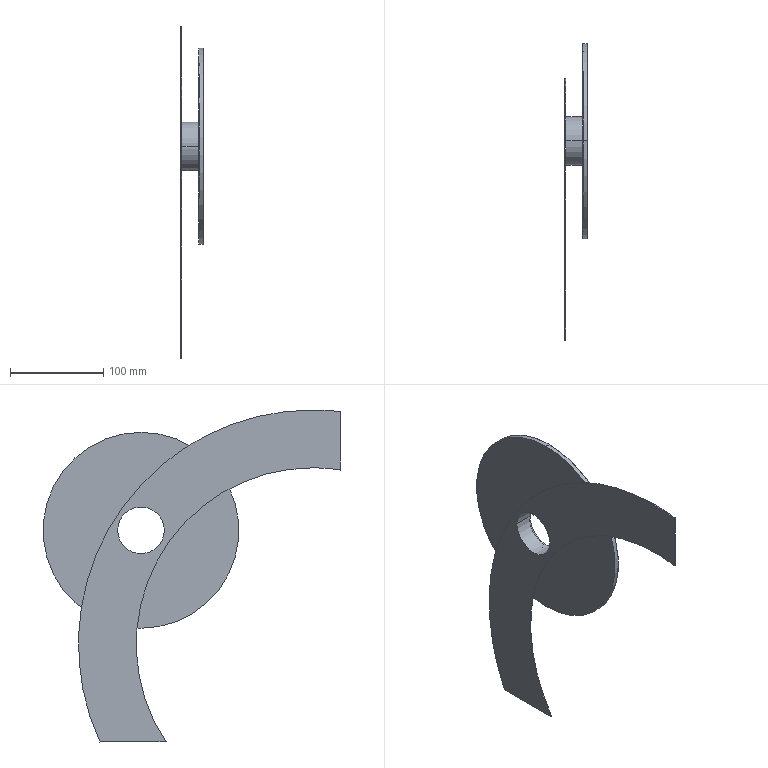Part | STEP file | 09-24 Track cover plate | 1 solid | 19 faces | box 24 x 319 x 356 mm | volume 66305 mm3 | cylinder 12 | plane 7 | commonest cylinder face diameters 50 x2 52 x2 208 x2 210 x2 378 x2 502 x2
STEP:
#1=CARTESIAN_POINT('',(0.,0.,0.));
#2=DIRECTION('',(0.,0.,1.));
#3=DIRECTION('',(1.,0.,0.));
#4=AXIS2_PLACEMENT_3D('',#1,#2,#3);
#5=CARTESIAN_POINT('',(24.,184.,226.));
#6=VERTEX_POINT('',#5);
#7=CARTESIAN_POINT('',(20.,184.,226.));
#8=VERTEX_POINT('',#7);
#9=CARTESIAN_POINT('',(24.,184.,226.));
#10=DIRECTION('',(-1.,0.,0.));
#11=VECTOR('',#10,1.);
#12=LINE('',#9,#11);
#13=CARTESIAN_POINT('',(24.,184.,122.));
#14=DIRECTION('',(-1.,0.,0.));
#15=DIRECTION('',(0.,0.,1.));
#16=AXIS2_PLACEMENT_3D('',#13,#14,#15);
#17=CYLINDRICAL_SURFACE('',#16,104.);
#18=CARTESIAN_POINT('',(6.283,0.));
#19=DIRECTION('',(0.,1.));
#20=VECTOR('',#19,1.);
#21=LINE('',#18,#20);
#22=(GEOMETRIC_REPRESENTATION_CONTEXT(2)PARAMETRIC_REPRESENTATION_CONTEXT()REPRESENTATION_CONTEXT('',''));
#23=DEFINITIONAL_REPRESENTATION('',(#21),#22);
#24=PCURVE('',#17,#23);
#25=CARTESIAN_POINT('',(24.,184.,122.));
#26=DIRECTION('',(-1.,0.,0.));
#27=DIRECTION('',(0.,0.,1.));
#28=AXIS2_PLACEMENT_3D('',#25,#26,#27);
#29=CYLINDRICAL_SURFACE('',#28,104.);
#30=CARTESIAN_POINT('',(0.,0.));
#31=DIRECTION('',(0.,1.));
#32=VECTOR('',#31,1.);
#33=LINE('',#30,#32);
#34=(GEOMETRIC_REPRESENTATION_CONTEXT(2)PARAMETRIC_REPRESENTATION_CONTEXT()REPRESENTATION_CONTEXT('',''));
#35=DEFINITIONAL_REPRESENTATION('',(#33),#34);
#36=PCURVE('',#29,#35);
#37=SURFACE_CURVE('',#12,(#24,#36),.PCURVE_S1.);
#38=EDGE_CURVE('',#6,#8,#37,.T.);
#39=ORIENTED_EDGE('',*,*,#38,.T.);
#40=CARTESIAN_POINT('',(20.,184.,18.));
#41=VERTEX_POINT('',#40);
#42=CARTESIAN_POINT('',(20.,184.,122.));
#43=DIRECTION('',(-1.,0.,0.));
#44=DIRECTION('',(0.,0.,1.));
#45=AXIS2_PLACEMENT_3D('',#42,#43,#44);
#46=CIRCLE('',#45,104.);
#47=CARTESIAN_POINT('',(0.,4.));
#48=DIRECTION('',(1.,0.));
#49=VECTOR('',#48,1.);
#50=LINE('',#47,#49);
#51=(GEOMETRIC_REPRESENTATION_CONTEXT(2)PARAMETRIC_REPRESENTATION_CONTEXT()REPRESENTATION_CONTEXT('',''));
#52=DEFINITIONAL_REPRESENTATION('',(#50),#51);
#53=PCURVE('',#17,#52);
#54=CARTESIAN_POINT('',(20.,78.752,227.248));
#55=DIRECTION('',(1.,0.,0.));
#56=DIRECTION('',(0.,0.,-1.));
#57=AXIS2_PLACEMENT_3D('',#54,#55,#56);
#58=PLANE('',#57);
#59=CARTESIAN_POINT('',(1.248,105.248));
#60=CARTESIAN_POINT('',(1.248,285.381));
#61=CARTESIAN_POINT('',(157.248,195.315));
#62=CARTESIAN_POINT('',(313.248,105.248));
#63=CARTESIAN_POINT('',(157.248,15.181));
#64=CARTESIAN_POINT('',(1.248,-74.885));
#65=CARTESIAN_POINT('',(1.248,105.248));
#66=(BOUNDED_CURVE()B_SPLINE_CURVE(2,(#59,#60,#61,#62,#63,#64,#65),.UNSPECIFIED.,.T.,.F.)B_SPLINE_CURVE_WITH_KNOTS((1,2,2,2,2,1),(-2.094,0.,2.094,4.189,6.283,8.378),.UNSPECIFIED.)CURVE()GEOMETRIC_REPRESENTATION_ITEM()RATIONAL_B_SPLINE_CURVE((1.,0.5,1.,0.5,1.,0.5,1.))REPRESENTATION_ITEM(''));
#67=(GEOMETRIC_REPRESENTATION_CONTEXT(2)PARAMETRIC_REPRESENTATION_CONTEXT()REPRESENTATION_CONTEXT('',''));
#68=DEFINITIONAL_REPRESENTATION('',(#66),#67);
#69=PCURVE('',#58,#68);
#70=SURFACE_CURVE('',#46,(#53,#69),.PCURVE_S1.);
#71=EDGE_CURVE('',#41,#8,#70,.T.);
#72=ORIENTED_EDGE('',*,*,#71,.F.);
#73=CARTESIAN_POINT('',(24.,184.,18.));
#74=VERTEX_POINT('',#73);
#75=CARTESIAN_POINT('',(24.,184.,18.));
#76=DIRECTION('',(-1.,0.,0.));
#77=VECTOR('',#76,1.);
#78=LINE('',#75,#77);
#79=CARTESIAN_POINT('',(3.142,0.));
#80=DIRECTION('',(0.,1.));
#81=VECTOR('',#80,1.);
#82=LINE('',#79,#81);
#83=(GEOMETRIC_REPRESENTATION_CONTEXT(2)PARAMETRIC_REPRESENTATION_CONTEXT()REPRESENTATION_CONTEXT('',''));
#84=DEFINITIONAL_REPRESENTATION('',(#82),#83);
#85=PCURVE('',#17,#84);
#86=CARTESIAN_POINT('',(3.142,0.));
#87=DIRECTION('',(0.,1.));
#88=VECTOR('',#87,1.);
#89=LINE('',#86,#88);
#90=(GEOMETRIC_REPRESENTATION_CONTEXT(2)PARAMETRIC_REPRESENTATION_CONTEXT()REPRESENTATION_CONTEXT('',''));
#91=DEFINITIONAL_REPRESENTATION('',(#89),#90);
#92=PCURVE('',#29,#91);
#93=SURFACE_CURVE('',#78,(#85,#92),.PCURVE_S1.);
#94=EDGE_CURVE('',#74,#41,#93,.T.);
#95=ORIENTED_EDGE('',*,*,#94,.F.);
#96=CARTESIAN_POINT('',(24.,184.,122.));
#97=DIRECTION('',(1.,0.,0.));
#98=DIRECTION('',(0.,0.,1.));
#99=AXIS2_PLACEMENT_3D('',#96,#97,#98);
#100=CIRCLE('',#99,104.);
#101=CARTESIAN_POINT('',(6.283,0.));
#102=DIRECTION('',(-1.,0.));
#103=VECTOR('',#102,1.);
#104=LINE('',#101,#103);
#105=(GEOMETRIC_REPRESENTATION_CONTEXT(2)PARAMETRIC_REPRESENTATION_CONTEXT()REPRESENTATION_CONTEXT('',''));
#106=DEFINITIONAL_REPRESENTATION('',(#104),#105);
#107=PCURVE('',#17,#106);
#108=CARTESIAN_POINT('',(24.,77.74,228.26));
#109=DIRECTION('',(1.,0.,0.));
#110=DIRECTION('',(0.,0.,-1.));
#111=AXIS2_PLACEMENT_3D('',#108,#109,#110);
#112=PLANE('',#111);
#113=CARTESIAN_POINT('',(106.26,106.26));
#114=DIRECTION('',(-1.,0.));
#115=AXIS2_PLACEMENT_2D('',#113,#114);
#116=CIRCLE('',#115,104.);
#117=(GEOMETRIC_REPRESENTATION_CONTEXT(2)PARAMETRIC_REPRESENTATION_CONTEXT()REPRESENTATION_CONTEXT('',''));
#118=DEFINITIONAL_REPRESENTATION('',(#116),#117);
#119=PCURVE('',#112,#118);
#120=SURFACE_CURVE('',#100,(#107,#119),.PCURVE_S1.);
#121=EDGE_CURVE('',#6,#74,#120,.T.);
#122=ORIENTED_EDGE('',*,*,#121,.F.);
#123=EDGE_LOOP('',(#39,#72,#95,#122));
#124=FACE_BOUND('',#123,.F.);
#125=ADVANCED_FACE('',(#124),#17,.F.);
#126=CARTESIAN_POINT('',(20.,159.,122.));
#127=VERTEX_POINT('',#126);
#128=CARTESIAN_POINT('',(0.,159.,122.));
#129=VERTEX_POINT('',#128);
#130=CARTESIAN_POINT('',(20.,159.,122.));
#131=DIRECTION('',(-1.,0.,0.));
#132=VECTOR('',#131,1.);
#133=LINE('',#130,#132);
#134=CARTESIAN_POINT('',(20.,184.,122.));
#135=DIRECTION('',(-1.,0.,0.));
#136=DIRECTION('',(0.,-1.,0.));
#137=AXIS2_PLACEMENT_3D('',#134,#135,#136);
#138=CYLINDRICAL_SURFACE('',#137,25.);
#139=CARTESIAN_POINT('',(6.283,0.));
#140=DIRECTION('',(0.,1.));
#141=VECTOR('',#140,1.);
#142=LINE('',#139,#141);
#143=(GEOMETRIC_REPRESENTATION_CONTEXT(2)PARAMETRIC_REPRESENTATION_CONTEXT()REPRESENTATION_CONTEXT('',''));
#144=DEFINITIONAL_REPRESENTATION('',(#142),#143);
#145=PCURVE('',#138,#144);
#146=CARTESIAN_POINT('',(20.,184.,122.));
#147=DIRECTION('',(-1.,0.,0.));
#148=DIRECTION('',(0.,-1.,0.));
#149=AXIS2_PLACEMENT_3D('',#146,#147,#148);
#150=CYLINDRICAL_SURFACE('',#149,25.);
#151=CARTESIAN_POINT('',(0.,0.));
#152=DIRECTION('',(0.,1.));
#153=VECTOR('',#152,1.);
#154=LINE('',#151,#153);
#155=(GEOMETRIC_REPRESENTATION_CONTEXT(2)PARAMETRIC_REPRESENTATION_CONTEXT()REPRESENTATION_CONTEXT('',''));
#156=DEFINITIONAL_REPRESENTATION('',(#154),#155);
#157=PCURVE('',#150,#156);
#158=SURFACE_CURVE('',#133,(#145,#157),.PCURVE_S1.);
#159=EDGE_CURVE('',#127,#129,#158,.T.);
#160=ORIENTED_EDGE('',*,*,#159,.T.);
#161=CARTESIAN_POINT('',(0.,209.,122.));
#162=VERTEX_POINT('',#161);
#163=CARTESIAN_POINT('',(0.,184.,122.));
#164=DIRECTION('',(-1.,0.,0.));
#165=DIRECTION('',(0.,-1.,0.));
#166=AXIS2_PLACEMENT_3D('',#163,#164,#165);
#167=CIRCLE('',#166,25.);
#168=CARTESIAN_POINT('',(0.,20.));
#169=DIRECTION('',(1.,0.));
#170=VECTOR('',#169,1.);
#171=LINE('',#168,#170);
#172=(GEOMETRIC_REPRESENTATION_CONTEXT(2)PARAMETRIC_REPRESENTATION_CONTEXT()REPRESENTATION_CONTEXT('',''));
#173=DEFINITIONAL_REPRESENTATION('',(#171),#172);
#174=PCURVE('',#138,#173);
#175=CARTESIAN_POINT('',(0.,-30.,253.136));
#176=DIRECTION('',(1.,0.,0.));
#177=DIRECTION('',(0.,0.,-1.));
#178=AXIS2_PLACEMENT_3D('',#175,#176,#177);
#179=PLANE('',#178);
#180=CARTESIAN_POINT('',(131.136,189.));
#181=CARTESIAN_POINT('',(87.835,189.));
#182=CARTESIAN_POINT('',(109.485,226.5));
#183=CARTESIAN_POINT('',(131.136,264.));
#184=CARTESIAN_POINT('',(152.787,226.5));
#185=CARTESIAN_POINT('',(174.437,189.));
#186=CARTESIAN_POINT('',(131.136,189.));
#187=(BOUNDED_CURVE()B_SPLINE_CURVE(2,(#180,#181,#182,#183,#184,#185,#186),.UNSPECIFIED.,.T.,.F.)B_SPLINE_CURVE_WITH_KNOTS((1,2,2,2,2,1),(-2.094,0.,2.094,4.189,6.283,8.378),.UNSPECIFIED.)CURVE()GEOMETRIC_REPRESENTATION_ITEM()RATIONAL_B_SPLINE_CURVE((1.,0.5,1.,0.5,1.,0.5,1.))REPRESENTATION_ITEM(''));
#188=(GEOMETRIC_REPRESENTATION_CONTEXT(2)PARAMETRIC_REPRESENTATION_CONTEXT()REPRESENTATION_CONTEXT('',''));
#189=DEFINITIONAL_REPRESENTATION('',(#187),#188);
#190=PCURVE('',#179,#189);
#191=SURFACE_CURVE('',#167,(#174,#190),.PCURVE_S1.);
#192=EDGE_CURVE('',#162,#129,#191,.T.);
#193=ORIENTED_EDGE('',*,*,#192,.F.);
#194=CARTESIAN_POINT('',(20.,209.,122.));
#195=VERTEX_POINT('',#194);
#196=CARTESIAN_POINT('',(20.,209.,122.));
#197=DIRECTION('',(-1.,0.,0.));
#198=VECTOR('',#197,1.);
#199=LINE('',#196,#198);
#200=CARTESIAN_POINT('',(3.142,0.));
#201=DIRECTION('',(0.,1.));
#202=VECTOR('',#201,1.);
#203=LINE('',#200,#202);
#204=(GEOMETRIC_REPRESENTATION_CONTEXT(2)PARAMETRIC_REPRESENTATION_CONTEXT()REPRESENTATION_CONTEXT('',''));
#205=DEFINITIONAL_REPRESENTATION('',(#203),#204);
#206=PCURVE('',#138,#205);
#207=CARTESIAN_POINT('',(3.142,0.));
#208=DIRECTION('',(0.,1.));
#209=VECTOR('',#208,1.);
#210=LINE('',#207,#209);
#211=(GEOMETRIC_REPRESENTATION_CONTEXT(2)PARAMETRIC_REPRESENTATION_CONTEXT()REPRESENTATION_CONTEXT('',''));
#212=DEFINITIONAL_REPRESENTATION('',(#210),#211);
#213=PCURVE('',#150,#212);
#214=SURFACE_CURVE('',#199,(#206,#213),.PCURVE_S1.);
#215=EDGE_CURVE('',#195,#162,#214,.T.);
#216=ORIENTED_EDGE('',*,*,#215,.F.);
#217=CARTESIAN_POINT('',(20.,184.,122.));
#218=DIRECTION('',(-1.,0.,0.));
#219=DIRECTION('',(0.,-1.,0.));
#220=AXIS2_PLACEMENT_3D('',#217,#218,#219);
#221=CIRCLE('',#220,25.);
#222=CARTESIAN_POINT('',(0.,0.));
#223=DIRECTION('',(1.,0.));
#224=VECTOR('',#223,1.);
#225=LINE('',#222,#224);
#226=(GEOMETRIC_REPRESENTATION_CONTEXT(2)PARAMETRIC_REPRESENTATION_CONTEXT()REPRESENTATION_CONTEXT('',''));
#227=DEFINITIONAL_REPRESENTATION('',(#225),#226);
#228=PCURVE('',#138,#227);
#229=CARTESIAN_POINT('',(105.248,80.248));
#230=CARTESIAN_POINT('',(61.947,80.248));
#231=CARTESIAN_POINT('',(83.597,117.748));
#232=CARTESIAN_POINT('',(105.248,155.248));
#233=CARTESIAN_POINT('',(126.899,117.748));
#234=CARTESIAN_POINT('',(148.549,80.248));
#235=CARTESIAN_POINT('',(105.248,80.248));
#236=(BOUNDED_CURVE()B_SPLINE_CURVE(2,(#229,#230,#231,#232,#233,#234,#235),.UNSPECIFIED.,.T.,.F.)B_SPLINE_CURVE_WITH_KNOTS((1,2,2,2,2,1),(-2.094,0.,2.094,4.189,6.283,8.378),.UNSPECIFIED.)CURVE()GEOMETRIC_REPRESENTATION_ITEM()RATIONAL_B_SPLINE_CURVE((1.,0.5,1.,0.5,1.,0.5,1.))REPRESENTATION_ITEM(''));
#237=(GEOMETRIC_REPRESENTATION_CONTEXT(2)PARAMETRIC_REPRESENTATION_CONTEXT()REPRESENTATION_CONTEXT('',''));
#238=DEFINITIONAL_REPRESENTATION('',(#236),#237);
#239=PCURVE('',#58,#238);
#240=SURFACE_CURVE('',#221,(#228,#239),.PCURVE_S1.);
#241=EDGE_CURVE('',#195,#127,#240,.T.);
#242=ORIENTED_EDGE('',*,*,#241,.T.);
#243=EDGE_LOOP('',(#160,#193,#216,#242));
#244=FACE_BOUND('',#243,.F.);
#245=ADVANCED_FACE('',(#244),#138,.F.);
#246=CARTESIAN_POINT('',(19.,184.,227.));
#247=VERTEX_POINT('',#246);
#248=CARTESIAN_POINT('',(19.,184.,17.));
#249=VERTEX_POINT('',#248);
#250=CARTESIAN_POINT('',(19.,184.,122.));
#251=DIRECTION('',(-1.,0.,0.));
#252=DIRECTION('',(0.,0.,-1.));
#253=AXIS2_PLACEMENT_3D('',#250,#251,#252);
#254=CIRCLE('',#253,105.);
#255=CARTESIAN_POINT('',(19.,184.,122.));
#256=DIRECTION('',(1.,0.,0.));
#257=DIRECTION('',(0.,0.,-1.));
#258=AXIS2_PLACEMENT_3D('',#255,#256,#257);
#259=CYLINDRICAL_SURFACE('',#258,105.);
#260=CARTESIAN_POINT('',(6.283,0.));
#261=DIRECTION('',(-1.,0.));
#262=VECTOR('',#261,1.);
#263=LINE('',#260,#262);
#264=(GEOMETRIC_REPRESENTATION_CONTEXT(2)PARAMETRIC_REPRESENTATION_CONTEXT()REPRESENTATION_CONTEXT('',''));
#265=DEFINITIONAL_REPRESENTATION('',(#263),#264);
#266=PCURVE('',#259,#265);
#267=CARTESIAN_POINT('',(19.,77.74,228.26));
#268=DIRECTION('',(1.,0.,0.));
#269=DIRECTION('',(0.,0.,-1.));
#270=AXIS2_PLACEMENT_3D('',#267,#268,#269);
#271=PLANE('',#270);
#272=CARTESIAN_POINT('',(211.26,106.26));
#273=CARTESIAN_POINT('',(211.26,-75.605));
#274=CARTESIAN_POINT('',(53.76,15.327));
#275=CARTESIAN_POINT('',(-103.74,106.26));
#276=CARTESIAN_POINT('',(53.76,197.193));
#277=CARTESIAN_POINT('',(211.26,288.125));
#278=CARTESIAN_POINT('',(211.26,106.26));
#279=(BOUNDED_CURVE()B_SPLINE_CURVE(2,(#272,#273,#274,#275,#276,#277,#278),.UNSPECIFIED.,.T.,.F.)B_SPLINE_CURVE_WITH_KNOTS((1,2,2,2,2,1),(-2.094,0.,2.094,4.189,6.283,8.378),.UNSPECIFIED.)CURVE()GEOMETRIC_REPRESENTATION_ITEM()RATIONAL_B_SPLINE_CURVE((1.,0.5,1.,0.5,1.,0.5,1.))REPRESENTATION_ITEM(''));
#280=(GEOMETRIC_REPRESENTATION_CONTEXT(2)PARAMETRIC_REPRESENTATION_CONTEXT()REPRESENTATION_CONTEXT('',''));
#281=DEFINITIONAL_REPRESENTATION('',(#279),#280);
#282=PCURVE('',#271,#281);
#283=SURFACE_CURVE('',#254,(#266,#282),.PCURVE_S1.);
#284=EDGE_CURVE('',#247,#249,#283,.T.);
#285=ORIENTED_EDGE('',*,*,#284,.F.);
#286=CARTESIAN_POINT('',(24.,184.,227.));
#287=VERTEX_POINT('',#286);
#288=CARTESIAN_POINT('',(19.,184.,227.));
#289=DIRECTION('',(1.,0.,0.));
#290=VECTOR('',#289,1.);
#291=LINE('',#288,#290);
#292=CARTESIAN_POINT('',(3.142,0.));
#293=DIRECTION('',(0.,1.));
#294=VECTOR('',#293,1.);
#295=LINE('',#292,#294);
#296=(GEOMETRIC_REPRESENTATION_CONTEXT(2)PARAMETRIC_REPRESENTATION_CONTEXT()REPRESENTATION_CONTEXT('',''));
#297=DEFINITIONAL_REPRESENTATION('',(#295),#296);
#298=PCURVE('',#259,#297);
#299=CARTESIAN_POINT('',(19.,184.,122.));
#300=DIRECTION('',(1.,0.,0.));
#301=DIRECTION('',(0.,0.,-1.));
#302=AXIS2_PLACEMENT_3D('',#299,#300,#301);
#303=CYLINDRICAL_SURFACE('',#302,105.);
#304=CARTESIAN_POINT('',(3.142,0.));
#305=DIRECTION('',(0.,1.));
#306=VECTOR('',#305,1.);
#307=LINE('',#304,#306);
#308=(GEOMETRIC_REPRESENTATION_CONTEXT(2)PARAMETRIC_REPRESENTATION_CONTEXT()REPRESENTATION_CONTEXT('',''));
#309=DEFINITIONAL_REPRESENTATION('',(#307),#308);
#310=PCURVE('',#303,#309);
#311=SURFACE_CURVE('',#291,(#298,#310),.PCURVE_S1.);
#312=EDGE_CURVE('',#247,#287,#311,.T.);
#313=ORIENTED_EDGE('',*,*,#312,.T.);
#314=CARTESIAN_POINT('',(24.,184.,17.));
#315=VERTEX_POINT('',#314);
#316=CARTESIAN_POINT('',(24.,184.,122.));
#317=DIRECTION('',(1.,0.,0.));
#318=DIRECTION('',(0.,0.,-1.));
#319=AXIS2_PLACEMENT_3D('',#316,#317,#318);
#320=CIRCLE('',#319,105.);
#321=CARTESIAN_POINT('',(0.,5.));
#322=DIRECTION('',(1.,0.));
#323=VECTOR('',#322,1.);
#324=LINE('',#321,#323);
#325=(GEOMETRIC_REPRESENTATION_CONTEXT(2)PARAMETRIC_REPRESENTATION_CONTEXT()REPRESENTATION_CONTEXT('',''));
#326=DEFINITIONAL_REPRESENTATION('',(#324),#325);
#327=PCURVE('',#259,#326);
#328=CARTESIAN_POINT('',(106.26,106.26));
#329=DIRECTION('',(1.,0.));
#330=AXIS2_PLACEMENT_2D('',#328,#329);
#331=CIRCLE('',#330,105.);
#332=(GEOMETRIC_REPRESENTATION_CONTEXT(2)PARAMETRIC_REPRESENTATION_CONTEXT()REPRESENTATION_CONTEXT('',''));
#333=DEFINITIONAL_REPRESENTATION('',(#331),#332);
#334=PCURVE('',#112,#333);
#335=SURFACE_CURVE('',#320,(#327,#334),.PCURVE_S1.);
#336=EDGE_CURVE('',#315,#287,#335,.T.);
#337=ORIENTED_EDGE('',*,*,#336,.F.);
#338=CARTESIAN_POINT('',(19.,184.,17.));
#339=DIRECTION('',(1.,0.,0.));
#340=VECTOR('',#339,1.);
#341=LINE('',#338,#340);
#342=CARTESIAN_POINT('',(0.,0.));
#343=DIRECTION('',(0.,1.));
#344=VECTOR('',#343,1.);
#345=LINE('',#342,#344);
#346=(GEOMETRIC_REPRESENTATION_CONTEXT(2)PARAMETRIC_REPRESENTATION_CONTEXT()REPRESENTATION_CONTEXT('',''));
#347=DEFINITIONAL_REPRESENTATION('',(#345),#346);
#348=PCURVE('',#259,#347);
#349=CARTESIAN_POINT('',(6.283,0.));
#350=DIRECTION('',(0.,1.));
#351=VECTOR('',#350,1.);
#352=LINE('',#349,#351);
#353=(GEOMETRIC_REPRESENTATION_CONTEXT(2)PARAMETRIC_REPRESENTATION_CONTEXT()REPRESENTATION_CONTEXT('',''));
#354=DEFINITIONAL_REPRESENTATION('',(#352),#353);
#355=PCURVE('',#303,#354);
#356=SURFACE_CURVE('',#341,(#348,#355),.PCURVE_S1.);
#357=EDGE_CURVE('',#249,#315,#356,.T.);
#358=ORIENTED_EDGE('',*,*,#357,.F.);
#359=EDGE_LOOP('',(#285,#313,#337,#358));
#360=FACE_BOUND('',#359,.T.);
#361=ADVANCED_FACE('',(#360),#259,.T.);
#362=CARTESIAN_POINT('',(1.,0.,251.));
#363=VERTEX_POINT('',#362);
#364=CARTESIAN_POINT('',(1.,-30.,249.201));
#365=VERTEX_POINT('',#364);
#366=CARTESIAN_POINT('',(1.,0.,0.));
#367=DIRECTION('',(1.,0.,0.));
#368=DIRECTION('',(0.,0.,1.));
#369=AXIS2_PLACEMENT_3D('',#366,#367,#368);
#370=CIRCLE('',#369,251.);
#371=CARTESIAN_POINT('',(1.,0.,0.));
#372=DIRECTION('',(-1.,0.,0.));
#373=DIRECTION('',(0.,0.,1.));
#374=AXIS2_PLACEMENT_3D('',#371,#372,#373);
#375=CYLINDRICAL_SURFACE('',#374,251.);
#376=CARTESIAN_POINT('',(6.283,0.));
#377=DIRECTION('',(-1.,0.));
#378=VECTOR('',#377,1.);
#379=LINE('',#376,#378);
#380=(GEOMETRIC_REPRESENTATION_CONTEXT(2)PARAMETRIC_REPRESENTATION_CONTEXT()REPRESENTATION_CONTEXT('',''));
#381=DEFINITIONAL_REPRESENTATION('',(#379),#380);
#382=PCURVE('',#375,#381);
#383=CARTESIAN_POINT('',(1.,-30.,253.136));
#384=DIRECTION('',(1.,0.,0.));
#385=DIRECTION('',(0.,0.,-1.));
#386=AXIS2_PLACEMENT_3D('',#383,#384,#385);
#387=PLANE('',#386);
#388=CARTESIAN_POINT('',(253.136,30.));
#389=DIRECTION('',(-1.,0.));
#390=AXIS2_PLACEMENT_2D('',#388,#389);
#391=CIRCLE('',#390,251.);
#392=(GEOMETRIC_REPRESENTATION_CONTEXT(2)PARAMETRIC_REPRESENTATION_CONTEXT()REPRESENTATION_CONTEXT('',''));
#393=DEFINITIONAL_REPRESENTATION('',(#391),#392);
#394=PCURVE('',#387,#393);
#395=SURFACE_CURVE('',#370,(#382,#394),.PCURVE_S1.);
#396=EDGE_CURVE('',#363,#365,#395,.T.);
#397=ORIENTED_EDGE('',*,*,#396,.F.);
#398=CARTESIAN_POINT('',(0.,0.,251.));
#399=VERTEX_POINT('',#398);
#400=CARTESIAN_POINT('',(1.,0.,251.));
#401=DIRECTION('',(-1.,0.,0.));
#402=VECTOR('',#401,1.);
#403=LINE('',#400,#402);
#404=CARTESIAN_POINT('',(6.283,0.));
#405=DIRECTION('',(0.,1.));
#406=VECTOR('',#405,1.);
#407=LINE('',#404,#406);
#408=(GEOMETRIC_REPRESENTATION_CONTEXT(2)PARAMETRIC_REPRESENTATION_CONTEXT()REPRESENTATION_CONTEXT('',''));
#409=DEFINITIONAL_REPRESENTATION('',(#407),#408);
#410=PCURVE('',#375,#409);
#411=CARTESIAN_POINT('',(1.,0.,0.));
#412=DIRECTION('',(-1.,0.,0.));
#413=DIRECTION('',(0.,0.,1.));
#414=AXIS2_PLACEMENT_3D('',#411,#412,#413);
#415=CYLINDRICAL_SURFACE('',#414,251.);
#416=CARTESIAN_POINT('',(0.,0.));
#417=DIRECTION('',(0.,1.));
#418=VECTOR('',#417,1.);
#419=LINE('',#416,#418);
#420=(GEOMETRIC_REPRESENTATION_CONTEXT(2)PARAMETRIC_REPRESENTATION_CONTEXT()REPRESENTATION_CONTEXT('',''));
#421=DEFINITIONAL_REPRESENTATION('',(#419),#420);
#422=PCURVE('',#415,#421);
#423=SURFACE_CURVE('',#403,(#410,#422),.PCURVE_S1.);
#424=EDGE_CURVE('',#363,#399,#423,.T.);
#425=ORIENTED_EDGE('',*,*,#424,.T.);
#426=CARTESIAN_POINT('',(0.,-30.,249.201));
#427=VERTEX_POINT('',#426);
#428=CARTESIAN_POINT('',(0.,0.,0.));
#429=DIRECTION('',(1.,0.,0.));
#430=DIRECTION('',(0.,0.,1.));
#431=AXIS2_PLACEMENT_3D('',#428,#429,#430);
#432=CIRCLE('',#431,251.);
#433=CARTESIAN_POINT('',(6.283,1.));
#434=DIRECTION('',(-1.,0.));
#435=VECTOR('',#434,1.);
#436=LINE('',#433,#435);
#437=(GEOMETRIC_REPRESENTATION_CONTEXT(2)PARAMETRIC_REPRESENTATION_CONTEXT()REPRESENTATION_CONTEXT('',''));
#438=DEFINITIONAL_REPRESENTATION('',(#436),#437);
#439=PCURVE('',#375,#438);
#440=CARTESIAN_POINT('',(253.136,30.));
#441=DIRECTION('',(-1.,0.));
#442=AXIS2_PLACEMENT_2D('',#440,#441);
#443=CIRCLE('',#442,251.);
#444=(GEOMETRIC_REPRESENTATION_CONTEXT(2)PARAMETRIC_REPRESENTATION_CONTEXT()REPRESENTATION_CONTEXT('',''));
#445=DEFINITIONAL_REPRESENTATION('',(#443),#444);
#446=PCURVE('',#179,#445);
#447=SURFACE_CURVE('',#432,(#439,#446),.PCURVE_S1.);
#448=EDGE_CURVE('',#399,#427,#447,.T.);
#449=ORIENTED_EDGE('',*,*,#448,.T.);
#450=CARTESIAN_POINT('',(0.5,-30.,249.201));
#451=DIRECTION('',(1.,0.,0.));
#452=VECTOR('',#451,1.);
#453=LINE('',#450,#452);
#454=CARTESIAN_POINT('',(6.163,0.5));
#455=DIRECTION('',(0.,-1.));
#456=VECTOR('',#455,1.);
#457=LINE('',#454,#456);
#458=(GEOMETRIC_REPRESENTATION_CONTEXT(2)PARAMETRIC_REPRESENTATION_CONTEXT()REPRESENTATION_CONTEXT('',''));
#459=DEFINITIONAL_REPRESENTATION('',(#457),#458);
#460=PCURVE('',#375,#459);
#461=CARTESIAN_POINT('',(0.,-30.,186.604));
#462=DIRECTION('',(0.,1.,0.));
#463=DIRECTION('',(0.,0.,1.));
#464=AXIS2_PLACEMENT_3D('',#461,#462,#463);
#465=PLANE('',#464);
#466=CARTESIAN_POINT('',(62.597,0.5));
#467=DIRECTION('',(0.,1.));
#468=VECTOR('',#467,1.);
#469=LINE('',#466,#468);
#470=(GEOMETRIC_REPRESENTATION_CONTEXT(2)PARAMETRIC_REPRESENTATION_CONTEXT()REPRESENTATION_CONTEXT('',''));
#471=DEFINITIONAL_REPRESENTATION('',(#469),#470);
#472=PCURVE('',#465,#471);
#473=SURFACE_CURVE('',#453,(#460,#472),.PCURVE_S1.);
#474=EDGE_CURVE('',#427,#365,#473,.T.);
#475=ORIENTED_EDGE('',*,*,#474,.T.);
#476=EDGE_LOOP('',(#397,#425,#449,#475));
#477=FACE_BOUND('',#476,.T.);
#478=ADVANCED_FACE('',(#477),#375,.T.);
#479=CARTESIAN_POINT('',(0.,157.15,-105.));
#480=VERTEX_POINT('',#479);
#481=CARTESIAN_POINT('',(1.,157.15,-105.));
#482=VERTEX_POINT('',#481);
#483=CARTESIAN_POINT('',(0.5,157.15,-105.));
#484=DIRECTION('',(1.,0.,0.));
#485=VECTOR('',#484,1.);
#486=LINE('',#483,#485);
#487=CARTESIAN_POINT('',(1.,0.,0.));
#488=DIRECTION('',(-1.,0.,0.));
#489=DIRECTION('',(0.,0.,1.));
#490=AXIS2_PLACEMENT_3D('',#487,#488,#489);
#491=CYLINDRICAL_SURFACE('',#490,189.);
#492=CARTESIAN_POINT('',(2.16,0.5));
#493=DIRECTION('',(0.,-1.));
#494=VECTOR('',#493,1.);
#495=LINE('',#492,#494);
#496=(GEOMETRIC_REPRESENTATION_CONTEXT(2)PARAMETRIC_REPRESENTATION_CONTEXT()REPRESENTATION_CONTEXT('',''));
#497=DEFINITIONAL_REPRESENTATION('',(#495),#496);
#498=PCURVE('',#491,#497);
#499=CARTESIAN_POINT('',(0.,157.15,-105.));
#500=DIRECTION('',(0.,0.,1.));
#501=DIRECTION('',(1.,0.,0.));
#502=AXIS2_PLACEMENT_3D('',#499,#500,#501);
#503=PLANE('',#502);
#504=CARTESIAN_POINT('',(0.5,0.));
#505=DIRECTION('',(1.,0.));
#506=VECTOR('',#505,1.);
#507=LINE('',#504,#506);
#508=(GEOMETRIC_REPRESENTATION_CONTEXT(2)PARAMETRIC_REPRESENTATION_CONTEXT()REPRESENTATION_CONTEXT('',''));
#509=DEFINITIONAL_REPRESENTATION('',(#507),#508);
#510=PCURVE('',#503,#509);
#511=SURFACE_CURVE('',#486,(#498,#510),.PCURVE_S1.);
#512=EDGE_CURVE('',#480,#482,#511,.T.);
#513=ORIENTED_EDGE('',*,*,#512,.F.);
#514=CARTESIAN_POINT('',(0.,0.,189.));
#515=VERTEX_POINT('',#514);
#516=CARTESIAN_POINT('',(0.,0.,0.));
#517=DIRECTION('',(-1.,0.,0.));
#518=DIRECTION('',(0.,0.,1.));
#519=AXIS2_PLACEMENT_3D('',#516,#517,#518);
#520=CIRCLE('',#519,189.);
#521=CARTESIAN_POINT('',(0.,1.));
#522=DIRECTION('',(1.,0.));
#523=VECTOR('',#522,1.);
#524=LINE('',#521,#523);
#525=(GEOMETRIC_REPRESENTATION_CONTEXT(2)PARAMETRIC_REPRESENTATION_CONTEXT()REPRESENTATION_CONTEXT('',''));
#526=DEFINITIONAL_REPRESENTATION('',(#524),#525);
#527=PCURVE('',#491,#526);
#528=CARTESIAN_POINT('',(64.136,30.));
#529=CARTESIAN_POINT('',(64.136,357.358));
#530=CARTESIAN_POINT('',(347.636,193.679));
#531=CARTESIAN_POINT('',(631.136,30.));
#532=CARTESIAN_POINT('',(347.636,-133.679));
#533=CARTESIAN_POINT('',(64.136,-297.358));
#534=CARTESIAN_POINT('',(64.136,30.));
#535=(BOUNDED_CURVE()B_SPLINE_CURVE(2,(#528,#529,#530,#531,#532,#533,#534),.UNSPECIFIED.,.T.,.F.)B_SPLINE_CURVE_WITH_KNOTS((1,2,2,2,2,1),(-2.094,0.,2.094,4.189,6.283,8.378),.UNSPECIFIED.)CURVE()GEOMETRIC_REPRESENTATION_ITEM()RATIONAL_B_SPLINE_CURVE((1.,0.5,1.,0.5,1.,0.5,1.))REPRESENTATION_ITEM(''));
#536=(GEOMETRIC_REPRESENTATION_CONTEXT(2)PARAMETRIC_REPRESENTATION_CONTEXT()REPRESENTATION_CONTEXT('',''));
#537=DEFINITIONAL_REPRESENTATION('',(#535),#536);
#538=PCURVE('',#179,#537);
#539=SURFACE_CURVE('',#520,(#527,#538),.PCURVE_S1.);
#540=EDGE_CURVE('',#515,#480,#539,.T.);
#541=ORIENTED_EDGE('',*,*,#540,.F.);
#542=CARTESIAN_POINT('',(1.,0.,189.));
#543=VERTEX_POINT('',#542);
#544=CARTESIAN_POINT('',(1.,0.,189.));
#545=DIRECTION('',(-1.,0.,0.));
#546=VECTOR('',#545,1.);
#547=LINE('',#544,#546);
#548=CARTESIAN_POINT('',(0.,0.));
#549=DIRECTION('',(0.,1.));
#550=VECTOR('',#549,1.);
#551=LINE('',#548,#550);
#552=(GEOMETRIC_REPRESENTATION_CONTEXT(2)PARAMETRIC_REPRESENTATION_CONTEXT()REPRESENTATION_CONTEXT('',''));
#553=DEFINITIONAL_REPRESENTATION('',(#551),#552);
#554=PCURVE('',#491,#553);
#555=CARTESIAN_POINT('',(1.,0.,0.));
#556=DIRECTION('',(-1.,0.,0.));
#557=DIRECTION('',(0.,0.,1.));
#558=AXIS2_PLACEMENT_3D('',#555,#556,#557);
#559=CYLINDRICAL_SURFACE('',#558,189.);
#560=CARTESIAN_POINT('',(6.283,0.));
#561=DIRECTION('',(0.,1.));
#562=VECTOR('',#561,1.);
#563=LINE('',#560,#562);
#564=(GEOMETRIC_REPRESENTATION_CONTEXT(2)PARAMETRIC_REPRESENTATION_CONTEXT()REPRESENTATION_CONTEXT('',''));
#565=DEFINITIONAL_REPRESENTATION('',(#563),#564);
#566=PCURVE('',#559,#565);
#567=SURFACE_CURVE('',#547,(#554,#566),.PCURVE_S1.);
#568=EDGE_CURVE('',#543,#515,#567,.T.);
#569=ORIENTED_EDGE('',*,*,#568,.F.);
#570=CARTESIAN_POINT('',(1.,0.,0.));
#571=DIRECTION('',(1.,0.,0.));
#572=DIRECTION('',(0.,0.,1.));
#573=AXIS2_PLACEMENT_3D('',#570,#571,#572);
#574=CIRCLE('',#573,189.);
#575=CARTESIAN_POINT('',(6.283,0.));
#576=DIRECTION('',(-1.,0.));
#577=VECTOR('',#576,1.);
#578=LINE('',#575,#577);
#579=(GEOMETRIC_REPRESENTATION_CONTEXT(2)PARAMETRIC_REPRESENTATION_CONTEXT()REPRESENTATION_CONTEXT('',''));
#580=DEFINITIONAL_REPRESENTATION('',(#578),#579);
#581=PCURVE('',#491,#580);
#582=CARTESIAN_POINT('',(253.136,30.));
#583=DIRECTION('',(-1.,0.));
#584=AXIS2_PLACEMENT_2D('',#582,#583);
#585=CIRCLE('',#584,189.);
#586=(GEOMETRIC_REPRESENTATION_CONTEXT(2)PARAMETRIC_REPRESENTATION_CONTEXT()REPRESENTATION_CONTEXT('',''));
#587=DEFINITIONAL_REPRESENTATION('',(#585),#586);
#588=PCURVE('',#387,#587);
#589=SURFACE_CURVE('',#574,(#581,#588),.PCURVE_S1.);
#590=EDGE_CURVE('',#482,#543,#589,.T.);
#591=ORIENTED_EDGE('',*,*,#590,.F.);
#592=EDGE_LOOP('',(#513,#541,#569,#591));
#593=FACE_BOUND('',#592,.F.);
#594=ADVANCED_FACE('',(#593),#491,.F.);
#595=CARTESIAN_POINT('',(19.,184.,148.));
#596=VERTEX_POINT('',#595);
#597=CARTESIAN_POINT('',(19.,184.,96.));
#598=VERTEX_POINT('',#597);
#599=CARTESIAN_POINT('',(19.,184.,122.));
#600=DIRECTION('',(-1.,0.,0.));
#601=DIRECTION('',(0.,0.,1.));
#602=AXIS2_PLACEMENT_3D('',#599,#600,#601);
#603=CIRCLE('',#602,26.);
#604=CARTESIAN_POINT('',(19.,184.,122.));
#605=DIRECTION('',(-1.,0.,0.));
#606=DIRECTION('',(0.,0.,1.));
#607=AXIS2_PLACEMENT_3D('',#604,#605,#606);
#608=CYLINDRICAL_SURFACE('',#607,26.);
#609=CARTESIAN_POINT('',(0.,0.));
#610=DIRECTION('',(1.,0.));
#611=VECTOR('',#610,1.);
#612=LINE('',#609,#611);
#613=(GEOMETRIC_REPRESENTATION_CONTEXT(2)PARAMETRIC_REPRESENTATION_CONTEXT()REPRESENTATION_CONTEXT('',''));
#614=DEFINITIONAL_REPRESENTATION('',(#612),#613);
#615=PCURVE('',#608,#614);
#616=CARTESIAN_POINT('',(80.26,106.26));
#617=CARTESIAN_POINT('',(80.26,151.293));
#618=CARTESIAN_POINT('',(119.26,128.777));
#619=CARTESIAN_POINT('',(158.26,106.26));
#620=CARTESIAN_POINT('',(119.26,83.743));
#621=CARTESIAN_POINT('',(80.26,61.227));
#622=CARTESIAN_POINT('',(80.26,106.26));
#623=(BOUNDED_CURVE()B_SPLINE_CURVE(2,(#616,#617,#618,#619,#620,#621,#622),.UNSPECIFIED.,.T.,.F.)B_SPLINE_CURVE_WITH_KNOTS((1,2,2,2,2,1),(-2.094,0.,2.094,4.189,6.283,8.378),.UNSPECIFIED.)CURVE()GEOMETRIC_REPRESENTATION_ITEM()RATIONAL_B_SPLINE_CURVE((1.,0.5,1.,0.5,1.,0.5,1.))REPRESENTATION_ITEM(''));
#624=(GEOMETRIC_REPRESENTATION_CONTEXT(2)PARAMETRIC_REPRESENTATION_CONTEXT()REPRESENTATION_CONTEXT('',''));
#625=DEFINITIONAL_REPRESENTATION('',(#623),#624);
#626=PCURVE('',#271,#625);
#627=SURFACE_CURVE('',#603,(#615,#626),.PCURVE_S1.);
#628=EDGE_CURVE('',#596,#598,#627,.T.);
#629=ORIENTED_EDGE('',*,*,#628,.T.);
#630=CARTESIAN_POINT('',(1.,184.,96.));
#631=VERTEX_POINT('',#630);
#632=CARTESIAN_POINT('',(19.,184.,96.));
#633=DIRECTION('',(-1.,0.,0.));
#634=VECTOR('',#633,1.);
#635=LINE('',#632,#634);
#636=CARTESIAN_POINT('',(3.142,0.));
#637=DIRECTION('',(0.,1.));
#638=VECTOR('',#637,1.);
#639=LINE('',#636,#638);
#640=(GEOMETRIC_REPRESENTATION_CONTEXT(2)PARAMETRIC_REPRESENTATION_CONTEXT()REPRESENTATION_CONTEXT('',''));
#641=DEFINITIONAL_REPRESENTATION('',(#639),#640);
#642=PCURVE('',#608,#641);
#643=CARTESIAN_POINT('',(19.,184.,122.));
#644=DIRECTION('',(-1.,0.,0.));
#645=DIRECTION('',(0.,0.,1.));
#646=AXIS2_PLACEMENT_3D('',#643,#644,#645);
#647=CYLINDRICAL_SURFACE('',#646,26.);
#648=CARTESIAN_POINT('',(3.142,0.));
#649=DIRECTION('',(0.,1.));
#650=VECTOR('',#649,1.);
#651=LINE('',#648,#650);
#652=(GEOMETRIC_REPRESENTATION_CONTEXT(2)PARAMETRIC_REPRESENTATION_CONTEXT()REPRESENTATION_CONTEXT('',''));
#653=DEFINITIONAL_REPRESENTATION('',(#651),#652);
#654=PCURVE('',#647,#653);
#655=SURFACE_CURVE('',#635,(#642,#654),.PCURVE_S1.);
#656=EDGE_CURVE('',#598,#631,#655,.T.);
#657=ORIENTED_EDGE('',*,*,#656,.T.);
#658=CARTESIAN_POINT('',(1.,184.,148.));
#659=VERTEX_POINT('',#658);
#660=CARTESIAN_POINT('',(1.,184.,122.));
#661=DIRECTION('',(-1.,0.,0.));
#662=DIRECTION('',(0.,0.,1.));
#663=AXIS2_PLACEMENT_3D('',#660,#661,#662);
#664=CIRCLE('',#663,26.);
#665=CARTESIAN_POINT('',(0.,18.));
#666=DIRECTION('',(1.,0.));
#667=VECTOR('',#666,1.);
#668=LINE('',#665,#667);
#669=(GEOMETRIC_REPRESENTATION_CONTEXT(2)PARAMETRIC_REPRESENTATION_CONTEXT()REPRESENTATION_CONTEXT('',''));
#670=DEFINITIONAL_REPRESENTATION('',(#668),#669);
#671=PCURVE('',#608,#670);
#672=CARTESIAN_POINT('',(105.136,214.));
#673=CARTESIAN_POINT('',(105.136,259.033));
#674=CARTESIAN_POINT('',(144.136,236.517));
#675=CARTESIAN_POINT('',(183.136,214.));
#676=CARTESIAN_POINT('',(144.136,191.483));
#677=CARTESIAN_POINT('',(105.136,168.967));
#678=CARTESIAN_POINT('',(105.136,214.));
#679=(BOUNDED_CURVE()B_SPLINE_CURVE(2,(#672,#673,#674,#675,#676,#677,#678),.UNSPECIFIED.,.T.,.F.)B_SPLINE_CURVE_WITH_KNOTS((1,2,2,2,2,1),(-2.094,0.,2.094,4.189,6.283,8.378),.UNSPECIFIED.)CURVE()GEOMETRIC_REPRESENTATION_ITEM()RATIONAL_B_SPLINE_CURVE((1.,0.5,1.,0.5,1.,0.5,1.))REPRESENTATION_ITEM(''));
#680=(GEOMETRIC_REPRESENTATION_CONTEXT(2)PARAMETRIC_REPRESENTATION_CONTEXT()REPRESENTATION_CONTEXT('',''));
#681=DEFINITIONAL_REPRESENTATION('',(#679),#680);
#682=PCURVE('',#387,#681);
#683=SURFACE_CURVE('',#664,(#671,#682),.PCURVE_S1.);
#684=EDGE_CURVE('',#659,#631,#683,.T.);
#685=ORIENTED_EDGE('',*,*,#684,.F.);
#686=CARTESIAN_POINT('',(19.,184.,148.));
#687=DIRECTION('',(-1.,0.,0.));
#688=VECTOR('',#687,1.);
#689=LINE('',#686,#688);
#690=CARTESIAN_POINT('',(0.,0.));
#691=DIRECTION('',(0.,1.));
#692=VECTOR('',#691,1.);
#693=LINE('',#690,#692);
#694=(GEOMETRIC_REPRESENTATION_CONTEXT(2)PARAMETRIC_REPRESENTATION_CONTEXT()REPRESENTATION_CONTEXT('',''));
#695=DEFINITIONAL_REPRESENTATION('',(#693),#694);
#696=PCURVE('',#608,#695);
#697=CARTESIAN_POINT('',(6.283,0.));
#698=DIRECTION('',(0.,1.));
#699=VECTOR('',#698,1.);
#700=LINE('',#697,#699);
#701=(GEOMETRIC_REPRESENTATION_CONTEXT(2)PARAMETRIC_REPRESENTATION_CONTEXT()REPRESENTATION_CONTEXT('',''));
#702=DEFINITIONAL_REPRESENTATION('',(#700),#701);
#703=PCURVE('',#647,#702);
#704=SURFACE_CURVE('',#689,(#696,#703),.PCURVE_S1.);
#705=EDGE_CURVE('',#596,#659,#704,.T.);
#706=ORIENTED_EDGE('',*,*,#705,.F.);
#707=EDGE_LOOP('',(#629,#657,#685,#706));
#708=FACE_BOUND('',#707,.T.);
#709=ADVANCED_FACE('',(#708),#608,.T.);
#710=CARTESIAN_POINT('',(20.,184.,122.));
#711=DIRECTION('',(-1.,0.,0.));
#712=DIRECTION('',(0.,0.,1.));
#713=AXIS2_PLACEMENT_3D('',#710,#711,#712);
#714=CIRCLE('',#713,104.);
#715=CARTESIAN_POINT('',(0.,4.));
#716=DIRECTION('',(1.,0.));
#717=VECTOR('',#716,1.);
#718=LINE('',#715,#717);
#719=(GEOMETRIC_REPRESENTATION_CONTEXT(2)PARAMETRIC_REPRESENTATION_CONTEXT()REPRESENTATION_CONTEXT('',''));
#720=DEFINITIONAL_REPRESENTATION('',(#718),#719);
#721=PCURVE('',#29,#720);
#722=CARTESIAN_POINT('',(1.248,105.248));
#723=CARTESIAN_POINT('',(1.248,285.381));
#724=CARTESIAN_POINT('',(157.248,195.315));
#725=CARTESIAN_POINT('',(313.248,105.248));
#726=CARTESIAN_POINT('',(157.248,15.181));
#727=CARTESIAN_POINT('',(1.248,-74.885));
#728=CARTESIAN_POINT('',(1.248,105.248));
#729=(BOUNDED_CURVE()B_SPLINE_CURVE(2,(#722,#723,#724,#725,#726,#727,#728),.UNSPECIFIED.,.T.,.F.)B_SPLINE_CURVE_WITH_KNOTS((1,2,2,2,2,1),(-2.094,0.,2.094,4.189,6.283,8.378),.UNSPECIFIED.)CURVE()GEOMETRIC_REPRESENTATION_ITEM()RATIONAL_B_SPLINE_CURVE((1.,0.5,1.,0.5,1.,0.5,1.))REPRESENTATION_ITEM(''));
#730=(GEOMETRIC_REPRESENTATION_CONTEXT(2)PARAMETRIC_REPRESENTATION_CONTEXT()REPRESENTATION_CONTEXT('',''));
#731=DEFINITIONAL_REPRESENTATION('',(#729),#730);
#732=PCURVE('',#58,#731);
#733=SURFACE_CURVE('',#714,(#721,#732),.PCURVE_S1.);
#734=EDGE_CURVE('',#8,#41,#733,.T.);
#735=ORIENTED_EDGE('',*,*,#734,.F.);
#736=ORIENTED_EDGE('',*,*,#38,.F.);
#737=CARTESIAN_POINT('',(24.,184.,122.));
#738=DIRECTION('',(1.,0.,0.));
#739=DIRECTION('',(0.,0.,1.));
#740=AXIS2_PLACEMENT_3D('',#737,#738,#739);
#741=CIRCLE('',#740,104.);
#742=CARTESIAN_POINT('',(6.283,0.));
#743=DIRECTION('',(-1.,0.));
#744=VECTOR('',#743,1.);
#745=LINE('',#742,#744);
#746=(GEOMETRIC_REPRESENTATION_CONTEXT(2)PARAMETRIC_REPRESENTATION_CONTEXT()REPRESENTATION_CONTEXT('',''));
#747=DEFINITIONAL_REPRESENTATION('',(#745),#746);
#748=PCURVE('',#29,#747);
#749=CARTESIAN_POINT('',(106.26,106.26));
#750=DIRECTION('',(-1.,0.));
#751=AXIS2_PLACEMENT_2D('',#749,#750);
#752=CIRCLE('',#751,104.);
#753=(GEOMETRIC_REPRESENTATION_CONTEXT(2)PARAMETRIC_REPRESENTATION_CONTEXT()REPRESENTATION_CONTEXT('',''));
#754=DEFINITIONAL_REPRESENTATION('',(#752),#753);
#755=PCURVE('',#112,#754);
#756=SURFACE_CURVE('',#741,(#748,#755),.PCURVE_S1.);
#757=EDGE_CURVE('',#74,#6,#756,.T.);
#758=ORIENTED_EDGE('',*,*,#757,.F.);
#759=ORIENTED_EDGE('',*,*,#94,.T.);
#760=EDGE_LOOP('',(#735,#736,#758,#759));
#761=FACE_BOUND('',#760,.F.);
#762=ADVANCED_FACE('',(#761),#29,.F.);
#763=CARTESIAN_POINT('',(20.,184.,122.));
#764=DIRECTION('',(-1.,0.,0.));
#765=DIRECTION('',(0.,-1.,0.));
#766=AXIS2_PLACEMENT_3D('',#763,#764,#765);
#767=CIRCLE('',#766,25.);
#768=CARTESIAN_POINT('',(105.248,80.248));
#769=CARTESIAN_POINT('',(61.947,80.248));
#770=CARTESIAN_POINT('',(83.597,117.748));
#771=CARTESIAN_POINT('',(105.248,155.248));
#772=CARTESIAN_POINT('',(126.899,117.748));
#773=CARTESIAN_POINT('',(148.549,80.248));
#774=CARTESIAN_POINT('',(105.248,80.248));
#775=(BOUNDED_CURVE()B_SPLINE_CURVE(2,(#768,#769,#770,#771,#772,#773,#774),.UNSPECIFIED.,.T.,.F.)B_SPLINE_CURVE_WITH_KNOTS((1,2,2,2,2,1),(-2.094,0.,2.094,4.189,6.283,8.378),.UNSPECIFIED.)CURVE()GEOMETRIC_REPRESENTATION_ITEM()RATIONAL_B_SPLINE_CURVE((1.,0.5,1.,0.5,1.,0.5,1.))REPRESENTATION_ITEM(''));
#776=(GEOMETRIC_REPRESENTATION_CONTEXT(2)PARAMETRIC_REPRESENTATION_CONTEXT()REPRESENTATION_CONTEXT('',''));
#777=DEFINITIONAL_REPRESENTATION('',(#775),#776);
#778=PCURVE('',#58,#777);
#779=CARTESIAN_POINT('',(0.,0.));
#780=DIRECTION('',(1.,0.));
#781=VECTOR('',#780,1.);
#782=LINE('',#779,#781);
#783=(GEOMETRIC_REPRESENTATION_CONTEXT(2)PARAMETRIC_REPRESENTATION_CONTEXT()REPRESENTATION_CONTEXT('',''));
#784=DEFINITIONAL_REPRESENTATION('',(#782),#783);
#785=PCURVE('',#150,#784);
#786=SURFACE_CURVE('',#767,(#778,#785),.PCURVE_S1.);
#787=EDGE_CURVE('',#127,#195,#786,.T.);
#788=ORIENTED_EDGE('',*,*,#787,.T.);
#789=ORIENTED_EDGE('',*,*,#241,.T.);
#790=EDGE_LOOP('',(#788,#789));
#791=FACE_BOUND('',#790,.T.);
#792=ORIENTED_EDGE('',*,*,#734,.F.);
#793=ORIENTED_EDGE('',*,*,#71,.F.);
#794=EDGE_LOOP('',(#792,#793));
#795=FACE_BOUND('',#794,.T.);
#796=ADVANCED_FACE('',(#791,#795),#58,.T.);
#797=ORIENTED_EDGE('',*,*,#121,.F.);
#798=ORIENTED_EDGE('',*,*,#757,.F.);
#799=EDGE_LOOP('',(#797,#798));
#800=FACE_BOUND('',#799,.T.);
#801=ORIENTED_EDGE('',*,*,#336,.T.);
#802=CARTESIAN_POINT('',(24.,184.,122.));
#803=DIRECTION('',(1.,0.,0.));
#804=DIRECTION('',(0.,0.,-1.));
#805=AXIS2_PLACEMENT_3D('',#802,#803,#804);
#806=CIRCLE('',#805,105.);
#807=CARTESIAN_POINT('',(106.26,106.26));
#808=DIRECTION('',(1.,0.));
#809=AXIS2_PLACEMENT_2D('',#807,#808);
#810=CIRCLE('',#809,105.);
#811=(GEOMETRIC_REPRESENTATION_CONTEXT(2)PARAMETRIC_REPRESENTATION_CONTEXT()REPRESENTATION_CONTEXT('',''));
#812=DEFINITIONAL_REPRESENTATION('',(#810),#811);
#813=PCURVE('',#112,#812);
#814=CARTESIAN_POINT('',(0.,5.));
#815=DIRECTION('',(1.,0.));
#816=VECTOR('',#815,1.);
#817=LINE('',#814,#816);
#818=(GEOMETRIC_REPRESENTATION_CONTEXT(2)PARAMETRIC_REPRESENTATION_CONTEXT()REPRESENTATION_CONTEXT('',''));
#819=DEFINITIONAL_REPRESENTATION('',(#817),#818);
#820=PCURVE('',#303,#819);
#821=SURFACE_CURVE('',#806,(#813,#820),.PCURVE_S1.);
#822=EDGE_CURVE('',#287,#315,#821,.T.);
#823=ORIENTED_EDGE('',*,*,#822,.T.);
#824=EDGE_LOOP('',(#801,#823));
#825=FACE_BOUND('',#824,.T.);
#826=ADVANCED_FACE('',(#800,#825),#112,.T.);
#827=CARTESIAN_POINT('',(0.,184.,122.));
#828=DIRECTION('',(-1.,0.,0.));
#829=DIRECTION('',(0.,-1.,0.));
#830=AXIS2_PLACEMENT_3D('',#827,#828,#829);
#831=CIRCLE('',#830,25.);
#832=CARTESIAN_POINT('',(0.,20.));
#833=DIRECTION('',(1.,0.));
#834=VECTOR('',#833,1.);
#835=LINE('',#832,#834);
#836=(GEOMETRIC_REPRESENTATION_CONTEXT(2)PARAMETRIC_REPRESENTATION_CONTEXT()REPRESENTATION_CONTEXT('',''));
#837=DEFINITIONAL_REPRESENTATION('',(#835),#836);
#838=PCURVE('',#150,#837);
#839=CARTESIAN_POINT('',(131.136,189.));
#840=CARTESIAN_POINT('',(87.835,189.));
#841=CARTESIAN_POINT('',(109.485,226.5));
#842=CARTESIAN_POINT('',(131.136,264.));
#843=CARTESIAN_POINT('',(152.787,226.5));
#844=CARTESIAN_POINT('',(174.437,189.));
#845=CARTESIAN_POINT('',(131.136,189.));
#846=(BOUNDED_CURVE()B_SPLINE_CURVE(2,(#839,#840,#841,#842,#843,#844,#845),.UNSPECIFIED.,.T.,.F.)B_SPLINE_CURVE_WITH_KNOTS((1,2,2,2,2,1),(-2.094,0.,2.094,4.189,6.283,8.378),.UNSPECIFIED.)CURVE()GEOMETRIC_REPRESENTATION_ITEM()RATIONAL_B_SPLINE_CURVE((1.,0.5,1.,0.5,1.,0.5,1.))REPRESENTATION_ITEM(''));
#847=(GEOMETRIC_REPRESENTATION_CONTEXT(2)PARAMETRIC_REPRESENTATION_CONTEXT()REPRESENTATION_CONTEXT('',''));
#848=DEFINITIONAL_REPRESENTATION('',(#846),#847);
#849=PCURVE('',#179,#848);
#850=SURFACE_CURVE('',#831,(#838,#849),.PCURVE_S1.);
#851=EDGE_CURVE('',#129,#162,#850,.T.);
#852=ORIENTED_EDGE('',*,*,#851,.F.);
#853=ORIENTED_EDGE('',*,*,#159,.F.);
#854=ORIENTED_EDGE('',*,*,#787,.T.);
#855=ORIENTED_EDGE('',*,*,#215,.T.);
#856=EDGE_LOOP('',(#852,#853,#854,#855));
#857=FACE_BOUND('',#856,.F.);
#858=ADVANCED_FACE('',(#857),#150,.F.);
#859=ORIENTED_EDGE('',*,*,#312,.F.);
#860=CARTESIAN_POINT('',(19.,184.,122.));
#861=DIRECTION('',(-1.,0.,0.));
#862=DIRECTION('',(0.,0.,-1.));
#863=AXIS2_PLACEMENT_3D('',#860,#861,#862);
#864=CIRCLE('',#863,105.);
#865=CARTESIAN_POINT('',(6.283,0.));
#866=DIRECTION('',(-1.,0.));
#867=VECTOR('',#866,1.);
#868=LINE('',#865,#867);
#869=(GEOMETRIC_REPRESENTATION_CONTEXT(2)PARAMETRIC_REPRESENTATION_CONTEXT()REPRESENTATION_CONTEXT('',''));
#870=DEFINITIONAL_REPRESENTATION('',(#868),#869);
#871=PCURVE('',#303,#870);
#872=CARTESIAN_POINT('',(211.26,106.26));
#873=CARTESIAN_POINT('',(211.26,-75.605));
#874=CARTESIAN_POINT('',(53.76,15.327));
#875=CARTESIAN_POINT('',(-103.74,106.26));
#876=CARTESIAN_POINT('',(53.76,197.193));
#877=CARTESIAN_POINT('',(211.26,288.125));
#878=CARTESIAN_POINT('',(211.26,106.26));
#879=(BOUNDED_CURVE()B_SPLINE_CURVE(2,(#872,#873,#874,#875,#876,#877,#878),.UNSPECIFIED.,.T.,.F.)B_SPLINE_CURVE_WITH_KNOTS((1,2,2,2,2,1),(-2.094,0.,2.094,4.189,6.283,8.378),.UNSPECIFIED.)CURVE()GEOMETRIC_REPRESENTATION_ITEM()RATIONAL_B_SPLINE_CURVE((1.,0.5,1.,0.5,1.,0.5,1.))REPRESENTATION_ITEM(''));
#880=(GEOMETRIC_REPRESENTATION_CONTEXT(2)PARAMETRIC_REPRESENTATION_CONTEXT()REPRESENTATION_CONTEXT('',''));
#881=DEFINITIONAL_REPRESENTATION('',(#879),#880);
#882=PCURVE('',#271,#881);
#883=SURFACE_CURVE('',#864,(#871,#882),.PCURVE_S1.);
#884=EDGE_CURVE('',#249,#247,#883,.T.);
#885=ORIENTED_EDGE('',*,*,#884,.F.);
#886=ORIENTED_EDGE('',*,*,#357,.T.);
#887=ORIENTED_EDGE('',*,*,#822,.F.);
#888=EDGE_LOOP('',(#859,#885,#886,#887));
#889=FACE_BOUND('',#888,.T.);
#890=ADVANCED_FACE('',(#889),#303,.T.);
#891=ORIENTED_EDGE('',*,*,#851,.F.);
#892=ORIENTED_EDGE('',*,*,#192,.F.);
#893=EDGE_LOOP('',(#891,#892));
#894=FACE_BOUND('',#893,.T.);
#895=CARTESIAN_POINT('',(0.,227.982,-105.));
#896=VERTEX_POINT('',#895);
#897=CARTESIAN_POINT('',(0.,111.343,-105.));
#898=DIRECTION('',(0.,1.,0.));
#899=VECTOR('',#898,1.);
#900=LINE('',#897,#899);
#901=CARTESIAN_POINT('',(358.136,141.343));
#902=DIRECTION('',(0.,1.));
#903=VECTOR('',#902,1.);
#904=LINE('',#901,#903);
#905=(GEOMETRIC_REPRESENTATION_CONTEXT(2)PARAMETRIC_REPRESENTATION_CONTEXT()REPRESENTATION_CONTEXT('',''));
#906=DEFINITIONAL_REPRESENTATION('',(#904),#905);
#907=PCURVE('',#179,#906);
#908=CARTESIAN_POINT('',(0.,-45.807));
#909=DIRECTION('',(0.,1.));
#910=VECTOR('',#909,1.);
#911=LINE('',#908,#910);
#912=(GEOMETRIC_REPRESENTATION_CONTEXT(2)PARAMETRIC_REPRESENTATION_CONTEXT()REPRESENTATION_CONTEXT('',''));
#913=DEFINITIONAL_REPRESENTATION('',(#911),#912);
#914=PCURVE('',#503,#913);
#915=SURFACE_CURVE('',#900,(#907,#914),.PCURVE_S1.);
#916=EDGE_CURVE('',#480,#896,#915,.T.);
#917=ORIENTED_EDGE('',*,*,#916,.F.);
#918=ORIENTED_EDGE('',*,*,#540,.F.);
#919=CARTESIAN_POINT('',(0.,-30.,186.604));
#920=VERTEX_POINT('',#919);
#921=CARTESIAN_POINT('',(0.,0.,0.));
#922=DIRECTION('',(-1.,0.,0.));
#923=DIRECTION('',(0.,0.,1.));
#924=AXIS2_PLACEMENT_3D('',#921,#922,#923);
#925=CIRCLE('',#924,189.);
#926=CARTESIAN_POINT('',(64.136,30.));
#927=CARTESIAN_POINT('',(64.136,357.358));
#928=CARTESIAN_POINT('',(347.636,193.679));
#929=CARTESIAN_POINT('',(631.136,30.));
#930=CARTESIAN_POINT('',(347.636,-133.679));
#931=CARTESIAN_POINT('',(64.136,-297.358));
#932=CARTESIAN_POINT('',(64.136,30.));
#933=(BOUNDED_CURVE()B_SPLINE_CURVE(2,(#926,#927,#928,#929,#930,#931,#932),.UNSPECIFIED.,.T.,.F.)B_SPLINE_CURVE_WITH_KNOTS((1,2,2,2,2,1),(-2.094,0.,2.094,4.189,6.283,8.378),.UNSPECIFIED.)CURVE()GEOMETRIC_REPRESENTATION_ITEM()RATIONAL_B_SPLINE_CURVE((1.,0.5,1.,0.5,1.,0.5,1.))REPRESENTATION_ITEM(''));
#934=(GEOMETRIC_REPRESENTATION_CONTEXT(2)PARAMETRIC_REPRESENTATION_CONTEXT()REPRESENTATION_CONTEXT('',''));
#935=DEFINITIONAL_REPRESENTATION('',(#933),#934);
#936=PCURVE('',#179,#935);
#937=CARTESIAN_POINT('',(0.,1.));
#938=DIRECTION('',(1.,0.));
#939=VECTOR('',#938,1.);
#940=LINE('',#937,#939);
#941=(GEOMETRIC_REPRESENTATION_CONTEXT(2)PARAMETRIC_REPRESENTATION_CONTEXT()REPRESENTATION_CONTEXT('',''));
#942=DEFINITIONAL_REPRESENTATION('',(#940),#941);
#943=PCURVE('',#559,#942);
#944=SURFACE_CURVE('',#925,(#936,#943),.PCURVE_S1.);
#945=EDGE_CURVE('',#920,#515,#944,.T.);
#946=ORIENTED_EDGE('',*,*,#945,.F.);
#947=CARTESIAN_POINT('',(0.,-30.,74.068));
#948=DIRECTION('',(0.,0.,-1.));
#949=VECTOR('',#948,1.);
#950=LINE('',#947,#949);
#951=CARTESIAN_POINT('',(179.068,0.));
#952=DIRECTION('',(1.,0.));
#953=VECTOR('',#952,1.);
#954=LINE('',#951,#953);
#955=(GEOMETRIC_REPRESENTATION_CONTEXT(2)PARAMETRIC_REPRESENTATION_CONTEXT()REPRESENTATION_CONTEXT('',''));
#956=DEFINITIONAL_REPRESENTATION('',(#954),#955);
#957=PCURVE('',#179,#956);
#958=CARTESIAN_POINT('',(-112.536,0.));
#959=DIRECTION('',(-1.,0.));
#960=VECTOR('',#959,1.);
#961=LINE('',#958,#960);
#962=(GEOMETRIC_REPRESENTATION_CONTEXT(2)PARAMETRIC_REPRESENTATION_CONTEXT()REPRESENTATION_CONTEXT('',''));
#963=DEFINITIONAL_REPRESENTATION('',(#961),#962);
#964=PCURVE('',#465,#963);
#965=SURFACE_CURVE('',#950,(#957,#964),.PCURVE_S1.);
#966=EDGE_CURVE('',#427,#920,#965,.T.);
#967=ORIENTED_EDGE('',*,*,#966,.F.);
#968=ORIENTED_EDGE('',*,*,#448,.F.);
#969=CARTESIAN_POINT('',(0.,0.,0.));
#970=DIRECTION('',(1.,0.,0.));
#971=DIRECTION('',(0.,0.,1.));
#972=AXIS2_PLACEMENT_3D('',#969,#970,#971);
#973=CIRCLE('',#972,251.);
#974=CARTESIAN_POINT('',(253.136,30.));
#975=DIRECTION('',(-1.,0.));
#976=AXIS2_PLACEMENT_2D('',#974,#975);
#977=CIRCLE('',#976,251.);
#978=(GEOMETRIC_REPRESENTATION_CONTEXT(2)PARAMETRIC_REPRESENTATION_CONTEXT()REPRESENTATION_CONTEXT('',''));
#979=DEFINITIONAL_REPRESENTATION('',(#977),#978);
#980=PCURVE('',#179,#979);
#981=CARTESIAN_POINT('',(6.283,1.));
#982=DIRECTION('',(-1.,0.));
#983=VECTOR('',#982,1.);
#984=LINE('',#981,#983);
#985=(GEOMETRIC_REPRESENTATION_CONTEXT(2)PARAMETRIC_REPRESENTATION_CONTEXT()REPRESENTATION_CONTEXT('',''));
#986=DEFINITIONAL_REPRESENTATION('',(#984),#985);
#987=PCURVE('',#415,#986);
#988=SURFACE_CURVE('',#973,(#980,#987),.PCURVE_S1.);
#989=EDGE_CURVE('',#896,#399,#988,.T.);
#990=ORIENTED_EDGE('',*,*,#989,.F.);
#991=EDGE_LOOP('',(#917,#918,#946,#967,#968,#990));
#992=FACE_BOUND('',#991,.T.);
#993=ADVANCED_FACE('',(#894,#992),#179,.F.);
#994=ORIENTED_EDGE('',*,*,#628,.F.);
#995=CARTESIAN_POINT('',(19.,184.,122.));
#996=DIRECTION('',(-1.,0.,0.));
#997=DIRECTION('',(0.,0.,1.));
#998=AXIS2_PLACEMENT_3D('',#995,#996,#997);
#999=CIRCLE('',#998,26.);
#1000=CARTESIAN_POINT('',(80.26,106.26));
#1001=CARTESIAN_POINT('',(80.26,151.293));
#1002=CARTESIAN_POINT('',(119.26,128.777));
#1003=CARTESIAN_POINT('',(158.26,106.26));
#1004=CARTESIAN_POINT('',(119.26,83.743));
#1005=CARTESIAN_POINT('',(80.26,61.227));
#1006=CARTESIAN_POINT('',(80.26,106.26));
#1007=(BOUNDED_CURVE()B_SPLINE_CURVE(2,(#1000,#1001,#1002,#1003,#1004,#1005,#1006),.UNSPECIFIED.,.T.,.F.)B_SPLINE_CURVE_WITH_KNOTS((1,2,2,2,2,1),(-2.094,0.,2.094,4.189,6.283,8.378),.UNSPECIFIED.)CURVE()GEOMETRIC_REPRESENTATION_ITEM()RATIONAL_B_SPLINE_CURVE((1.,0.5,1.,0.5,1.,0.5,1.))REPRESENTATION_ITEM(''));
#1008=(GEOMETRIC_REPRESENTATION_CONTEXT(2)PARAMETRIC_REPRESENTATION_CONTEXT()REPRESENTATION_CONTEXT('',''));
#1009=DEFINITIONAL_REPRESENTATION('',(#1007),#1008);
#1010=PCURVE('',#271,#1009);
#1011=CARTESIAN_POINT('',(0.,0.));
#1012=DIRECTION('',(1.,0.));
#1013=VECTOR('',#1012,1.);
#1014=LINE('',#1011,#1013);
#1015=(GEOMETRIC_REPRESENTATION_CONTEXT(2)PARAMETRIC_REPRESENTATION_CONTEXT()REPRESENTATION_CONTEXT('',''));
#1016=DEFINITIONAL_REPRESENTATION('',(#1014),#1015);
#1017=PCURVE('',#647,#1016);
#1018=SURFACE_CURVE('',#999,(#1010,#1017),.PCURVE_S1.);
#1019=EDGE_CURVE('',#598,#596,#1018,.T.);
#1020=ORIENTED_EDGE('',*,*,#1019,.F.);
#1021=EDGE_LOOP('',(#994,#1020));
#1022=FACE_BOUND('',#1021,.T.);
#1023=ORIENTED_EDGE('',*,*,#884,.T.);
#1024=ORIENTED_EDGE('',*,*,#284,.T.);
#1025=EDGE_LOOP('',(#1023,#1024));
#1026=FACE_BOUND('',#1025,.T.);
#1027=ADVANCED_FACE('',(#1022,#1026),#271,.F.);
#1028=ORIENTED_EDGE('',*,*,#424,.F.);
#1029=CARTESIAN_POINT('',(1.,227.982,-105.));
#1030=VERTEX_POINT('',#1029);
#1031=CARTESIAN_POINT('',(1.,0.,0.));
#1032=DIRECTION('',(1.,0.,0.));
#1033=DIRECTION('',(0.,0.,1.));
#1034=AXIS2_PLACEMENT_3D('',#1031,#1032,#1033);
#1035=CIRCLE('',#1034,251.);
#1036=CARTESIAN_POINT('',(6.283,0.));
#1037=DIRECTION('',(-1.,0.));
#1038=VECTOR('',#1037,1.);
#1039=LINE('',#1036,#1038);
#1040=(GEOMETRIC_REPRESENTATION_CONTEXT(2)PARAMETRIC_REPRESENTATION_CONTEXT()REPRESENTATION_CONTEXT('',''));
#1041=DEFINITIONAL_REPRESENTATION('',(#1039),#1040);
#1042=PCURVE('',#415,#1041);
#1043=CARTESIAN_POINT('',(253.136,30.));
#1044=DIRECTION('',(-1.,0.));
#1045=AXIS2_PLACEMENT_2D('',#1043,#1044);
#1046=CIRCLE('',#1045,251.);
#1047=(GEOMETRIC_REPRESENTATION_CONTEXT(2)PARAMETRIC_REPRESENTATION_CONTEXT()REPRESENTATION_CONTEXT('',''));
#1048=DEFINITIONAL_REPRESENTATION('',(#1046),#1047);
#1049=PCURVE('',#387,#1048);
#1050=SURFACE_CURVE('',#1035,(#1042,#1049),.PCURVE_S1.);
#1051=EDGE_CURVE('',#1030,#363,#1050,.T.);
#1052=ORIENTED_EDGE('',*,*,#1051,.F.);
#1053=CARTESIAN_POINT('',(0.5,227.982,-105.));
#1054=DIRECTION('',(1.,0.,0.));
#1055=VECTOR('',#1054,1.);
#1056=LINE('',#1053,#1055);
#1057=CARTESIAN_POINT('',(2.002,0.5));
#1058=DIRECTION('',(0.,-1.));
#1059=VECTOR('',#1058,1.);
#1060=LINE('',#1057,#1059);
#1061=(GEOMETRIC_REPRESENTATION_CONTEXT(2)PARAMETRIC_REPRESENTATION_CONTEXT()REPRESENTATION_CONTEXT('',''));
#1062=DEFINITIONAL_REPRESENTATION('',(#1060),#1061);
#1063=PCURVE('',#415,#1062);
#1064=CARTESIAN_POINT('',(0.5,70.833));
#1065=DIRECTION('',(1.,0.));
#1066=VECTOR('',#1065,1.);
#1067=LINE('',#1064,#1066);
#1068=(GEOMETRIC_REPRESENTATION_CONTEXT(2)PARAMETRIC_REPRESENTATION_CONTEXT()REPRESENTATION_CONTEXT('',''));
#1069=DEFINITIONAL_REPRESENTATION('',(#1067),#1068);
#1070=PCURVE('',#503,#1069);
#1071=SURFACE_CURVE('',#1056,(#1063,#1070),.PCURVE_S1.);
#1072=EDGE_CURVE('',#896,#1030,#1071,.T.);
#1073=ORIENTED_EDGE('',*,*,#1072,.F.);
#1074=ORIENTED_EDGE('',*,*,#989,.T.);
#1075=EDGE_LOOP('',(#1028,#1052,#1073,#1074));
#1076=FACE_BOUND('',#1075,.T.);
#1077=ADVANCED_FACE('',(#1076),#415,.T.);
#1078=ORIENTED_EDGE('',*,*,#1072,.T.);
#1079=CARTESIAN_POINT('',(1.,192.566,-105.));
#1080=DIRECTION('',(0.,1.,0.));
#1081=VECTOR('',#1080,1.);
#1082=LINE('',#1079,#1081);
#1083=CARTESIAN_POINT('',(1.,35.416));
#1084=DIRECTION('',(0.,1.));
#1085=VECTOR('',#1084,1.);
#1086=LINE('',#1083,#1085);
#1087=(GEOMETRIC_REPRESENTATION_CONTEXT(2)PARAMETRIC_REPRESENTATION_CONTEXT()REPRESENTATION_CONTEXT('',''));
#1088=DEFINITIONAL_REPRESENTATION('',(#1086),#1087);
#1089=PCURVE('',#503,#1088);
#1090=CARTESIAN_POINT('',(358.136,222.566));
#1091=DIRECTION('',(0.,1.));
#1092=VECTOR('',#1091,1.);
#1093=LINE('',#1090,#1092);
#1094=(GEOMETRIC_REPRESENTATION_CONTEXT(2)PARAMETRIC_REPRESENTATION_CONTEXT()REPRESENTATION_CONTEXT('',''));
#1095=DEFINITIONAL_REPRESENTATION('',(#1093),#1094);
#1096=PCURVE('',#387,#1095);
#1097=SURFACE_CURVE('',#1082,(#1089,#1096),.PCURVE_S1.);
#1098=EDGE_CURVE('',#482,#1030,#1097,.T.);
#1099=ORIENTED_EDGE('',*,*,#1098,.F.);
#1100=ORIENTED_EDGE('',*,*,#512,.F.);
#1101=ORIENTED_EDGE('',*,*,#916,.T.);
#1102=EDGE_LOOP('',(#1078,#1099,#1100,#1101));
#1103=FACE_BOUND('',#1102,.T.);
#1104=ADVANCED_FACE('',(#1103),#503,.F.);
#1105=ORIENTED_EDGE('',*,*,#945,.F.);
#1106=CARTESIAN_POINT('',(1.,-30.,186.604));
#1107=VERTEX_POINT('',#1106);
#1108=CARTESIAN_POINT('',(0.5,-30.,186.604));
#1109=DIRECTION('',(-1.,0.,0.));
#1110=VECTOR('',#1109,1.);
#1111=LINE('',#1108,#1110);
#1112=CARTESIAN_POINT('',(6.124,0.5));
#1113=DIRECTION('',(0.,1.));
#1114=VECTOR('',#1113,1.);
#1115=LINE('',#1112,#1114);
#1116=(GEOMETRIC_REPRESENTATION_CONTEXT(2)PARAMETRIC_REPRESENTATION_CONTEXT()REPRESENTATION_CONTEXT('',''));
#1117=DEFINITIONAL_REPRESENTATION('',(#1115),#1116);
#1118=PCURVE('',#559,#1117);
#1119=CARTESIAN_POINT('',(0.000000011,0.5));
#1120=DIRECTION('',(0.,-1.));
#1121=VECTOR('',#1120,1.);
#1122=LINE('',#1119,#1121);
#1123=(GEOMETRIC_REPRESENTATION_CONTEXT(2)PARAMETRIC_REPRESENTATION_CONTEXT()REPRESENTATION_CONTEXT('',''));
#1124=DEFINITIONAL_REPRESENTATION('',(#1122),#1123);
#1125=PCURVE('',#465,#1124);
#1126=SURFACE_CURVE('',#1111,(#1118,#1125),.PCURVE_S1.);
#1127=EDGE_CURVE('',#1107,#920,#1126,.T.);
#1128=ORIENTED_EDGE('',*,*,#1127,.F.);
#1129=CARTESIAN_POINT('',(1.,0.,0.));
#1130=DIRECTION('',(1.,0.,0.));
#1131=DIRECTION('',(0.,0.,1.));
#1132=AXIS2_PLACEMENT_3D('',#1129,#1130,#1131);
#1133=CIRCLE('',#1132,189.);
#1134=CARTESIAN_POINT('',(6.283,0.));
#1135=DIRECTION('',(-1.,0.));
#1136=VECTOR('',#1135,1.);
#1137=LINE('',#1134,#1136);
#1138=(GEOMETRIC_REPRESENTATION_CONTEXT(2)PARAMETRIC_REPRESENTATION_CONTEXT()REPRESENTATION_CONTEXT('',''));
#1139=DEFINITIONAL_REPRESENTATION('',(#1137),#1138);
#1140=PCURVE('',#559,#1139);
#1141=CARTESIAN_POINT('',(253.136,30.));
#1142=DIRECTION('',(-1.,0.));
#1143=AXIS2_PLACEMENT_2D('',#1141,#1142);
#1144=CIRCLE('',#1143,189.);
#1145=(GEOMETRIC_REPRESENTATION_CONTEXT(2)PARAMETRIC_REPRESENTATION_CONTEXT()REPRESENTATION_CONTEXT('',''));
#1146=DEFINITIONAL_REPRESENTATION('',(#1144),#1145);
#1147=PCURVE('',#387,#1146);
#1148=SURFACE_CURVE('',#1133,(#1140,#1147),.PCURVE_S1.);
#1149=EDGE_CURVE('',#543,#1107,#1148,.T.);
#1150=ORIENTED_EDGE('',*,*,#1149,.F.);
#1151=ORIENTED_EDGE('',*,*,#568,.T.);
#1152=EDGE_LOOP('',(#1105,#1128,#1150,#1151));
#1153=FACE_BOUND('',#1152,.F.);
#1154=ADVANCED_FACE('',(#1153),#559,.F.);
#1155=ORIENTED_EDGE('',*,*,#1127,.F.);
#1156=CARTESIAN_POINT('',(1.,-30.,217.902));
#1157=DIRECTION('',(0.,0.,-1.));
#1158=VECTOR('',#1157,1.);
#1159=LINE('',#1156,#1158);
#1160=CARTESIAN_POINT('',(31.298,1.));
#1161=DIRECTION('',(-1.,0.));
#1162=VECTOR('',#1161,1.);
#1163=LINE('',#1160,#1162);
#1164=(GEOMETRIC_REPRESENTATION_CONTEXT(2)PARAMETRIC_REPRESENTATION_CONTEXT()REPRESENTATION_CONTEXT('',''));
#1165=DEFINITIONAL_REPRESENTATION('',(#1163),#1164);
#1166=PCURVE('',#465,#1165);
#1167=CARTESIAN_POINT('',(35.234,0.));
#1168=DIRECTION('',(1.,0.));
#1169=VECTOR('',#1168,1.);
#1170=LINE('',#1167,#1169);
#1171=(GEOMETRIC_REPRESENTATION_CONTEXT(2)PARAMETRIC_REPRESENTATION_CONTEXT()REPRESENTATION_CONTEXT('',''));
#1172=DEFINITIONAL_REPRESENTATION('',(#1170),#1171);
#1173=PCURVE('',#387,#1172);
#1174=SURFACE_CURVE('',#1159,(#1166,#1173),.PCURVE_S1.);
#1175=EDGE_CURVE('',#365,#1107,#1174,.T.);
#1176=ORIENTED_EDGE('',*,*,#1175,.F.);
#1177=ORIENTED_EDGE('',*,*,#474,.F.);
#1178=ORIENTED_EDGE('',*,*,#966,.T.);
#1179=EDGE_LOOP('',(#1155,#1176,#1177,#1178));
#1180=FACE_BOUND('',#1179,.T.);
#1181=ADVANCED_FACE('',(#1180),#465,.F.);
#1182=ORIENTED_EDGE('',*,*,#656,.F.);
#1183=ORIENTED_EDGE('',*,*,#1019,.T.);
#1184=ORIENTED_EDGE('',*,*,#705,.T.);
#1185=CARTESIAN_POINT('',(1.,184.,122.));
#1186=DIRECTION('',(-1.,0.,0.));
#1187=DIRECTION('',(0.,0.,1.));
#1188=AXIS2_PLACEMENT_3D('',#1185,#1186,#1187);
#1189=CIRCLE('',#1188,26.);
#1190=CARTESIAN_POINT('',(0.,18.));
#1191=DIRECTION('',(1.,0.));
#1192=VECTOR('',#1191,1.);
#1193=LINE('',#1190,#1192);
#1194=(GEOMETRIC_REPRESENTATION_CONTEXT(2)PARAMETRIC_REPRESENTATION_CONTEXT()REPRESENTATION_CONTEXT('',''));
#1195=DEFINITIONAL_REPRESENTATION('',(#1193),#1194);
#1196=PCURVE('',#647,#1195);
#1197=CARTESIAN_POINT('',(105.136,214.));
#1198=CARTESIAN_POINT('',(105.136,259.033));
#1199=CARTESIAN_POINT('',(144.136,236.517));
#1200=CARTESIAN_POINT('',(183.136,214.));
#1201=CARTESIAN_POINT('',(144.136,191.483));
#1202=CARTESIAN_POINT('',(105.136,168.967));
#1203=CARTESIAN_POINT('',(105.136,214.));
#1204=(BOUNDED_CURVE()B_SPLINE_CURVE(2,(#1197,#1198,#1199,#1200,#1201,#1202,#1203),.UNSPECIFIED.,.T.,.F.)B_SPLINE_CURVE_WITH_KNOTS((1,2,2,2,2,1),(-2.094,0.,2.094,4.189,6.283,8.378),.UNSPECIFIED.)CURVE()GEOMETRIC_REPRESENTATION_ITEM()RATIONAL_B_SPLINE_CURVE((1.,0.5,1.,0.5,1.,0.5,1.))REPRESENTATION_ITEM(''));
#1205=(GEOMETRIC_REPRESENTATION_CONTEXT(2)PARAMETRIC_REPRESENTATION_CONTEXT()REPRESENTATION_CONTEXT('',''));
#1206=DEFINITIONAL_REPRESENTATION('',(#1204),#1205);
#1207=PCURVE('',#387,#1206);
#1208=SURFACE_CURVE('',#1189,(#1196,#1207),.PCURVE_S1.);
#1209=EDGE_CURVE('',#631,#659,#1208,.T.);
#1210=ORIENTED_EDGE('',*,*,#1209,.F.);
#1211=EDGE_LOOP('',(#1182,#1183,#1184,#1210));
#1212=FACE_BOUND('',#1211,.T.);
#1213=ADVANCED_FACE('',(#1212),#647,.T.);
#1214=ORIENTED_EDGE('',*,*,#684,.T.);
#1215=ORIENTED_EDGE('',*,*,#1209,.T.);
#1216=EDGE_LOOP('',(#1214,#1215));
#1217=FACE_BOUND('',#1216,.T.);
#1218=ORIENTED_EDGE('',*,*,#590,.F.);
#1219=ORIENTED_EDGE('',*,*,#1098,.T.);
#1220=ORIENTED_EDGE('',*,*,#1051,.T.);
#1221=ORIENTED_EDGE('',*,*,#396,.T.);
#1222=ORIENTED_EDGE('',*,*,#1175,.T.);
#1223=ORIENTED_EDGE('',*,*,#1149,.F.);
#1224=EDGE_LOOP('',(#1218,#1219,#1220,#1221,#1222,#1223));
#1225=FACE_BOUND('',#1224,.T.);
#1226=ADVANCED_FACE('',(#1217,#1225),#387,.T.);
#1227=CLOSED_SHELL('',(#125,#245,#361,#478,#594,#709,#762,#796,#826,#858,#890,#993,#1027,#1077,#1104,#1154,#1181,#1213,#1226));
#1228=MANIFOLD_SOLID_BREP('',#1227);
#1229=(LENGTH_UNIT()NAMED_UNIT(*)SI_UNIT(.MILLI.,.METRE.));
#1230=UNCERTAINTY_MEASURE_WITH_UNIT(LENGTH_MEASURE(0.0000001),#1229,'','');
#1231=(NAMED_UNIT(*)PLANE_ANGLE_UNIT()SI_UNIT($,.RADIAN.));
#1232=(NAMED_UNIT(*)SI_UNIT($,.STERADIAN.)SOLID_ANGLE_UNIT());
#1233=(GEOMETRIC_REPRESENTATION_CONTEXT(3)GLOBAL_UNCERTAINTY_ASSIGNED_CONTEXT((#1230))GLOBAL_UNIT_ASSIGNED_CONTEXT((#1229,#1231,#1232))REPRESENTATION_CONTEXT('',''));
#1234=ADVANCED_BREP_SHAPE_REPRESENTATION('',(#4,#1228),#1233);